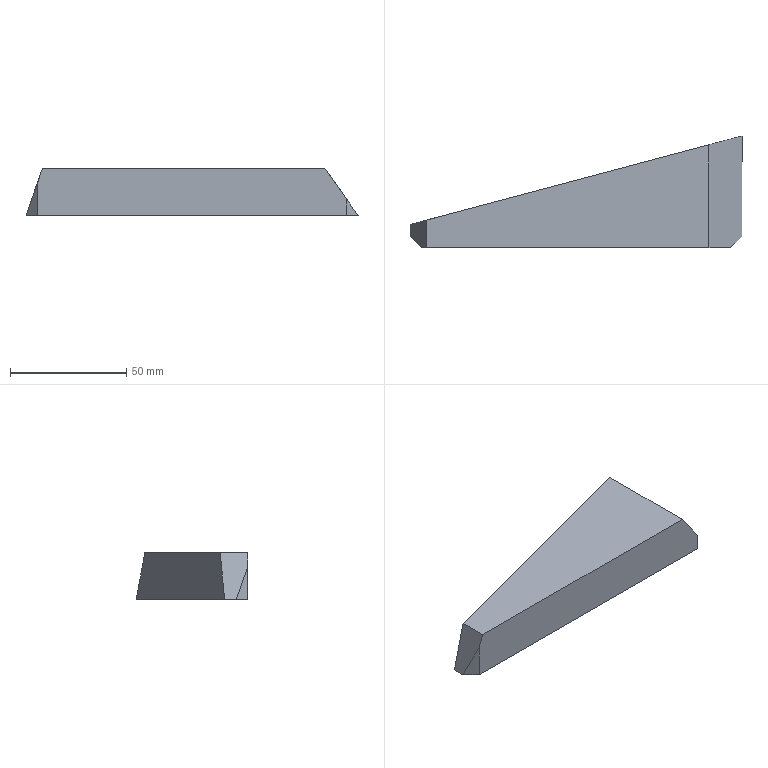Part | SolidWorks | features Extrusion 1, ICE 1 | 1 solid | 8 faces | box 142.6 x 48 x 20 mm | volume 75242 mm3 | plane 8
STEP:
#1=CARTESIAN_POINT('',(5.,0.,14.177));
#2=VERTEX_POINT('',#1);
#3=CARTESIAN_POINT('',(5.,0.,0.));
#4=VERTEX_POINT('',#3);
#5=CARTESIAN_POINT('',(5.,0.,20.));
#6=DIRECTION('',(0.,0.,-1.));
#7=VECTOR('',#6,1000.);
#8=LINE('',#5,#7);
#9=EDGE_CURVE('',#2,#4,#8,.T.);
#10=ORIENTED_EDGE('',*,*,#9,.F.);
#11=CARTESIAN_POINT('',(0.,5.,0.));
#12=VERTEX_POINT('',#11);
#13=CARTESIAN_POINT('',(5.649,-0.6486,16.016));
#14=DIRECTION('',(-0.3156,0.3156,-0.8949));
#15=VECTOR('',#14,1000.);
#16=LINE('',#13,#15);
#17=EDGE_CURVE('',#2,#12,#16,.T.);
#18=ORIENTED_EDGE('',*,*,#17,.T.);
#19=CARTESIAN_POINT('',(0.,5.,0.));
#20=DIRECTION('',(0.7071,-0.7071,0.));
#21=VECTOR('',#20,1000.);
#22=LINE('',#19,#21);
#23=EDGE_CURVE('',#12,#4,#22,.T.);
#24=ORIENTED_EDGE('',*,*,#23,.T.);
#25=EDGE_LOOP('',(#10,#18,#24));
#26=FACE_OUTER_BOUND('',#25,.T.);
#27=CARTESIAN_POINT('',(0.,5.,20.));
#28=DIRECTION('',(0.7071,0.7071,0.));
#29=DIRECTION('',(-0.7071,0.7071,0.));
#30=AXIS2_PLACEMENT_3D('',#27,#28,#29);
#31=PLANE('',#30);
#32=ADVANCED_FACE('',(#26),#31,.F.);
#33=CARTESIAN_POINT('',(137.6,0.,7.051));
#34=VERTEX_POINT('',#33);
#35=CARTESIAN_POINT('',(137.6,0.,0.));
#36=VERTEX_POINT('',#35);
#37=CARTESIAN_POINT('',(137.6,0.,20.));
#38=DIRECTION('',(0.,0.,-1.));
#39=VECTOR('',#38,1000.);
#40=LINE('',#37,#39);
#41=EDGE_CURVE('',#34,#36,#40,.T.);
#42=ORIENTED_EDGE('',*,*,#41,.F.);
#43=CARTESIAN_POINT('',(128.419,0.,20.));
#44=VERTEX_POINT('',#43);
#45=CARTESIAN_POINT('',(87.127,0.,78.234));
#46=DIRECTION('',(-0.5784,0.,0.8157));
#47=VECTOR('',#46,1000.);
#48=LINE('',#45,#47);
#49=EDGE_CURVE('',#34,#44,#48,.T.);
#50=ORIENTED_EDGE('',*,*,#49,.T.);
#51=CARTESIAN_POINT('',(7.054,0.,20.));
#52=VERTEX_POINT('',#51);
#53=CARTESIAN_POINT('',(5.,0.,20.));
#54=DIRECTION('',(1.,0.,0.));
#55=VECTOR('',#54,1000.);
#56=LINE('',#53,#55);
#57=EDGE_CURVE('',#52,#44,#56,.T.);
#58=ORIENTED_EDGE('',*,*,#57,.F.);
#59=CARTESIAN_POINT('',(6.827,0.,19.356));
#60=DIRECTION('',(-0.3326,0.,-0.9431));
#61=VECTOR('',#60,1000.);
#62=LINE('',#59,#61);
#63=EDGE_CURVE('',#52,#2,#62,.T.);
#64=ORIENTED_EDGE('',*,*,#63,.T.);
#65=ORIENTED_EDGE('',*,*,#9,.T.);
#66=CARTESIAN_POINT('',(5.,0.,0.));
#67=DIRECTION('',(1.,0.,0.));
#68=VECTOR('',#67,1000.);
#69=LINE('',#66,#68);
#70=EDGE_CURVE('',#4,#36,#69,.T.);
#71=ORIENTED_EDGE('',*,*,#70,.T.);
#72=EDGE_LOOP('',(#42,#50,#58,#64,#65,#71));
#73=FACE_OUTER_BOUND('',#72,.T.);
#74=CARTESIAN_POINT('',(5.,0.,20.));
#75=DIRECTION('',(0.,1.,0.));
#76=DIRECTION('',(0.,0.,1.));
#77=AXIS2_PLACEMENT_3D('',#74,#75,#76);
#78=PLANE('',#77);
#79=ADVANCED_FACE('',(#73),#78,.F.);
#80=CARTESIAN_POINT('',(142.6,5.,0.));
#81=VERTEX_POINT('',#80);
#82=CARTESIAN_POINT('',(137.6,0.,0.));
#83=DIRECTION('',(0.7071,0.7071,0.));
#84=VECTOR('',#83,1000.);
#85=LINE('',#82,#84);
#86=EDGE_CURVE('',#36,#81,#85,.T.);
#87=ORIENTED_EDGE('',*,*,#86,.T.);
#88=CARTESIAN_POINT('',(133.022,-4.578,13.508));
#89=DIRECTION('',(-0.5007,-0.5007,0.7061));
#90=VECTOR('',#89,1000.);
#91=LINE('',#88,#90);
#92=EDGE_CURVE('',#81,#34,#91,.T.);
#93=ORIENTED_EDGE('',*,*,#92,.T.);
#94=ORIENTED_EDGE('',*,*,#41,.T.);
#95=EDGE_LOOP('',(#87,#93,#94));
#96=FACE_OUTER_BOUND('',#95,.T.);
#97=CARTESIAN_POINT('',(137.6,0.,20.));
#98=DIRECTION('',(-0.7071,0.7071,0.));
#99=DIRECTION('',(-0.7071,-0.7071,0.));
#100=AXIS2_PLACEMENT_3D('',#97,#98,#99);
#101=PLANE('',#100);
#102=ADVANCED_FACE('',(#96),#101,.F.);
#103=CARTESIAN_POINT('',(128.419,44.221,20.));
#104=VERTEX_POINT('',#103);
#105=CARTESIAN_POINT('',(7.054,11.88,20.));
#106=VERTEX_POINT('',#105);
#107=CARTESIAN_POINT('',(142.6,48.,20.));
#108=DIRECTION('',(-0.9663,-0.2575,0.));
#109=VECTOR('',#108,1000.);
#110=LINE('',#107,#109);
#111=EDGE_CURVE('',#104,#106,#110,.T.);
#112=ORIENTED_EDGE('',*,*,#111,.F.);
#113=CARTESIAN_POINT('',(142.6,48.,0.));
#114=VERTEX_POINT('',#113);
#115=CARTESIAN_POINT('',(142.6,48.,0.));
#116=DIRECTION('',(-0.5717,-0.1523,0.8062));
#117=VECTOR('',#116,1000.);
#118=LINE('',#115,#117);
#119=EDGE_CURVE('',#114,#104,#118,.T.);
#120=ORIENTED_EDGE('',*,*,#119,.F.);
#121=CARTESIAN_POINT('',(0.,10.,0.));
#122=VERTEX_POINT('',#121);
#123=CARTESIAN_POINT('',(142.6,48.,0.));
#124=DIRECTION('',(-0.9663,-0.2575,0.));
#125=VECTOR('',#124,1000.);
#126=LINE('',#123,#125);
#127=EDGE_CURVE('',#114,#122,#126,.T.);
#128=ORIENTED_EDGE('',*,*,#127,.T.);
#129=CARTESIAN_POINT('',(0.,10.,0.));
#130=DIRECTION('',(-0.3313,-0.08829,-0.9394));
#131=VECTOR('',#130,1000.);
#132=LINE('',#129,#131);
#133=EDGE_CURVE('',#106,#122,#132,.T.);
#134=ORIENTED_EDGE('',*,*,#133,.F.);
#135=EDGE_LOOP('',(#112,#120,#128,#134));
#136=FACE_OUTER_BOUND('',#135,.T.);
#137=CARTESIAN_POINT('',(142.6,48.,20.));
#138=DIRECTION('',(0.2575,-0.9663,0.));
#139=DIRECTION('',(0.9663,0.2575,0.));
#140=AXIS2_PLACEMENT_3D('',#137,#138,#139);
#141=PLANE('',#140);
#142=ADVANCED_FACE('',(#136),#141,.F.);
#143=CARTESIAN_POINT('',(128.419,-5.779,20.));
#144=DIRECTION('',(0.,1.,0.));
#145=VECTOR('',#144,1000.);
#146=LINE('',#143,#145);
#147=EDGE_CURVE('',#44,#104,#146,.T.);
#148=ORIENTED_EDGE('',*,*,#147,.T.);
#149=ORIENTED_EDGE('',*,*,#111,.T.);
#150=CARTESIAN_POINT('',(7.054,-38.12,20.));
#151=DIRECTION('',(0.,1.,0.));
#152=VECTOR('',#151,1000.);
#153=LINE('',#150,#152);
#154=EDGE_CURVE('',#52,#106,#153,.T.);
#155=ORIENTED_EDGE('',*,*,#154,.F.);
#156=ORIENTED_EDGE('',*,*,#57,.T.);
#157=EDGE_LOOP('',(#148,#149,#155,#156));
#158=FACE_OUTER_BOUND('',#157,.T.);
#159=CARTESIAN_POINT('',(0.,0.,20.));
#160=DIRECTION('',(0.,0.,1.));
#161=DIRECTION('',(1.,0.,0.));
#162=AXIS2_PLACEMENT_3D('',#159,#160,#161);
#163=PLANE('',#162);
#164=ADVANCED_FACE('',(#158),#163,.T.);
#165=CARTESIAN_POINT('',(0.,10.,0.));
#166=DIRECTION('',(0.,-1.,0.));
#167=VECTOR('',#166,1000.);
#168=LINE('',#165,#167);
#169=EDGE_CURVE('',#122,#12,#168,.T.);
#170=ORIENTED_EDGE('',*,*,#169,.F.);
#171=ORIENTED_EDGE('',*,*,#127,.F.);
#172=CARTESIAN_POINT('',(142.6,5.,0.));
#173=DIRECTION('',(0.,1.,0.));
#174=VECTOR('',#173,1000.);
#175=LINE('',#172,#174);
#176=EDGE_CURVE('',#81,#114,#175,.T.);
#177=ORIENTED_EDGE('',*,*,#176,.F.);
#178=ORIENTED_EDGE('',*,*,#86,.F.);
#179=ORIENTED_EDGE('',*,*,#70,.F.);
#180=ORIENTED_EDGE('',*,*,#23,.F.);
#181=EDGE_LOOP('',(#170,#171,#177,#178,#179,#180));
#182=FACE_OUTER_BOUND('',#181,.T.);
#183=CARTESIAN_POINT('',(0.,0.,0.));
#184=DIRECTION('',(0.,0.,1.));
#185=DIRECTION('',(1.,0.,0.));
#186=AXIS2_PLACEMENT_3D('',#183,#184,#185);
#187=PLANE('',#186);
#188=ADVANCED_FACE('',(#182),#187,.F.);
#189=ORIENTED_EDGE('',*,*,#63,.F.);
#190=ORIENTED_EDGE('',*,*,#154,.T.);
#191=ORIENTED_EDGE('',*,*,#133,.T.);
#192=ORIENTED_EDGE('',*,*,#169,.T.);
#193=ORIENTED_EDGE('',*,*,#17,.F.);
#194=EDGE_LOOP('',(#189,#190,#191,#192,#193));
#195=FACE_OUTER_BOUND('',#194,.T.);
#196=CARTESIAN_POINT('',(0.,-40.,0.));
#197=DIRECTION('',(0.9431,0.,-0.3326));
#198=DIRECTION('',(-0.3326,0.,-0.9431));
#199=AXIS2_PLACEMENT_3D('',#196,#197,#198);
#200=PLANE('',#199);
#201=ADVANCED_FACE('',(#195),#200,.F.);
#202=ORIENTED_EDGE('',*,*,#92,.F.);
#203=ORIENTED_EDGE('',*,*,#176,.T.);
#204=ORIENTED_EDGE('',*,*,#119,.T.);
#205=ORIENTED_EDGE('',*,*,#147,.F.);
#206=ORIENTED_EDGE('',*,*,#49,.F.);
#207=EDGE_LOOP('',(#202,#203,#204,#205,#206));
#208=FACE_OUTER_BOUND('',#207,.T.);
#209=CARTESIAN_POINT('',(142.6,-2.,0.));
#210=DIRECTION('',(-0.8157,0.,-0.5784));
#211=DIRECTION('',(-0.5784,0.,0.8157));
#212=AXIS2_PLACEMENT_3D('',#209,#210,#211);
#213=PLANE('',#212);
#214=ADVANCED_FACE('',(#208),#213,.F.);
#215=CLOSED_SHELL('',(#32,#79,#102,#142,#164,#188,#201,#214));
#216=MANIFOLD_SOLID_BREP('',#215);
#217=CARTESIAN_POINT('',(0.,0.,0.));
#218=DIRECTION('',(0.,0.,1.));
#219=DIRECTION('',(1.,0.,0.));
#220=AXIS2_PLACEMENT_3D('',#217,#218,#219);
#221=(LENGTH_UNIT()NAMED_UNIT(*)SI_UNIT(.MILLI.,.METRE.));
#222=UNCERTAINTY_MEASURE_WITH_UNIT(LENGTH_MEASURE(0.00001),#221,'','');
#223=(NAMED_UNIT(*)PLANE_ANGLE_UNIT()SI_UNIT($,.RADIAN.));
#224=(NAMED_UNIT(*)SI_UNIT($,.STERADIAN.)SOLID_ANGLE_UNIT());
#225=(GEOMETRIC_REPRESENTATION_CONTEXT(3)GLOBAL_UNCERTAINTY_ASSIGNED_CONTEXT((#222))GLOBAL_UNIT_ASSIGNED_CONTEXT((#221,#223,#224))REPRESENTATION_CONTEXT('',''));
#226=ADVANCED_BREP_SHAPE_REPRESENTATION('',(#216,#220),#225);